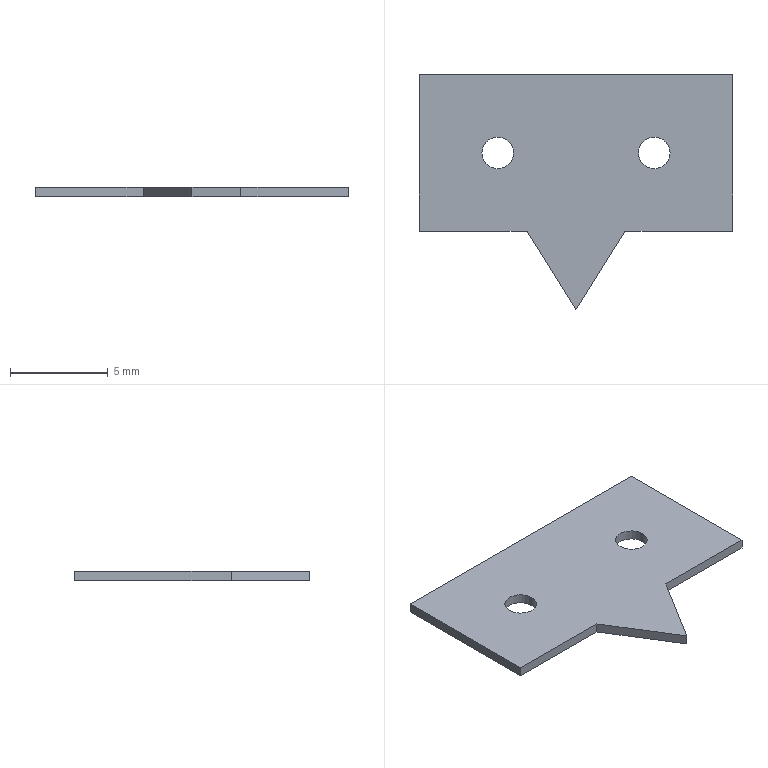Part | STEP file | 0232_012_PPS12 | 1 solid | 13 faces | box 16 x 12 x 0.5 mm | volume 66.945 mm3 | plane 9 | cylinder 4 | commonest cylinder face diameters 1.618 x4
STEP:
#1=CARTESIAN_POINT('',(0.,0.,0.));
#2=DIRECTION('',(0.,0.,1.));
#3=DIRECTION('',(1.,0.,0.));
#4=AXIS2_PLACEMENT_3D('',#1,#2,#3);
#5=CARTESIAN_POINT('',(-3.191,-4.,0.));
#6=VERTEX_POINT('',#5);
#7=CARTESIAN_POINT('',(-3.191,-4.,0.5));
#8=VERTEX_POINT('',#7);
#9=CARTESIAN_POINT('',(-3.191,-4.,0.));
#10=DIRECTION('',(0.,0.,1.));
#11=VECTOR('',#10,1.);
#12=LINE('',#9,#11);
#13=CARTESIAN_POINT('',(-4.,-4.,0.));
#14=DIRECTION('',(0.,0.,1.));
#15=DIRECTION('',(1.,0.,0.));
#16=AXIS2_PLACEMENT_3D('',#13,#14,#15);
#17=CYLINDRICAL_SURFACE('',#16,0.8088);
#18=CARTESIAN_POINT('',(6.283,0.));
#19=DIRECTION('',(0.,1.));
#20=VECTOR('',#19,1.);
#21=LINE('',#18,#20);
#22=(GEOMETRIC_REPRESENTATION_CONTEXT(2)PARAMETRIC_REPRESENTATION_CONTEXT()REPRESENTATION_CONTEXT('',''));
#23=DEFINITIONAL_REPRESENTATION('',(#21),#22);
#24=PCURVE('',#17,#23);
#25=CARTESIAN_POINT('',(-4.,-4.,0.));
#26=DIRECTION('',(0.,0.,1.));
#27=DIRECTION('',(1.,0.,0.));
#28=AXIS2_PLACEMENT_3D('',#25,#26,#27);
#29=CYLINDRICAL_SURFACE('',#28,0.8088);
#30=CARTESIAN_POINT('',(0.,0.));
#31=DIRECTION('',(0.,1.));
#32=VECTOR('',#31,1.);
#33=LINE('',#30,#32);
#34=(GEOMETRIC_REPRESENTATION_CONTEXT(2)PARAMETRIC_REPRESENTATION_CONTEXT()REPRESENTATION_CONTEXT('',''));
#35=DEFINITIONAL_REPRESENTATION('',(#33),#34);
#36=PCURVE('',#29,#35);
#37=SURFACE_CURVE('',#12,(#24,#36),.PCURVE_S1.);
#38=EDGE_CURVE('',#6,#8,#37,.T.);
#39=ORIENTED_EDGE('',*,*,#38,.T.);
#40=CARTESIAN_POINT('',(-4.809,-4.,0.5));
#41=VERTEX_POINT('',#40);
#42=CARTESIAN_POINT('',(-4.,-4.,0.5));
#43=DIRECTION('',(0.,0.,-1.));
#44=DIRECTION('',(1.,0.,0.));
#45=AXIS2_PLACEMENT_3D('',#42,#43,#44);
#46=CIRCLE('',#45,0.8088);
#47=CARTESIAN_POINT('',(6.283,0.5));
#48=DIRECTION('',(-1.,0.));
#49=VECTOR('',#48,1.);
#50=LINE('',#47,#49);
#51=(GEOMETRIC_REPRESENTATION_CONTEXT(2)PARAMETRIC_REPRESENTATION_CONTEXT()REPRESENTATION_CONTEXT('',''));
#52=DEFINITIONAL_REPRESENTATION('',(#50),#51);
#53=PCURVE('',#17,#52);
#54=CARTESIAN_POINT('',(0.,-4.698,0.5));
#55=DIRECTION('',(0.,0.,1.));
#56=DIRECTION('',(1.,0.,0.));
#57=AXIS2_PLACEMENT_3D('',#54,#55,#56);
#58=PLANE('',#57);
#59=CARTESIAN_POINT('',(-3.191,0.6981));
#60=CARTESIAN_POINT('',(-3.191,-0.7028));
#61=CARTESIAN_POINT('',(-4.404,-0.002343));
#62=CARTESIAN_POINT('',(-5.618,0.6981));
#63=CARTESIAN_POINT('',(-4.404,1.399));
#64=CARTESIAN_POINT('',(-3.191,2.099));
#65=CARTESIAN_POINT('',(-3.191,0.6981));
#66=(BOUNDED_CURVE()B_SPLINE_CURVE(2,(#59,#60,#61,#62,#63,#64,#65),.UNSPECIFIED.,.T.,.F.)B_SPLINE_CURVE_WITH_KNOTS((1,2,2,2,2,1),(-2.094,0.,2.094,4.189,6.283,8.378),.UNSPECIFIED.)CURVE()GEOMETRIC_REPRESENTATION_ITEM()RATIONAL_B_SPLINE_CURVE((1.,0.5,1.,0.5,1.,0.5,1.))REPRESENTATION_ITEM(''));
#67=(GEOMETRIC_REPRESENTATION_CONTEXT(2)PARAMETRIC_REPRESENTATION_CONTEXT()REPRESENTATION_CONTEXT('',''));
#68=DEFINITIONAL_REPRESENTATION('',(#66),#67);
#69=PCURVE('',#58,#68);
#70=SURFACE_CURVE('',#46,(#53,#69),.PCURVE_S1.);
#71=EDGE_CURVE('',#8,#41,#70,.T.);
#72=ORIENTED_EDGE('',*,*,#71,.T.);
#73=CARTESIAN_POINT('',(-4.809,-4.,0.));
#74=VERTEX_POINT('',#73);
#75=CARTESIAN_POINT('',(-4.809,-4.,0.));
#76=DIRECTION('',(0.,0.,1.));
#77=VECTOR('',#76,1.);
#78=LINE('',#75,#77);
#79=CARTESIAN_POINT('',(3.142,0.));
#80=DIRECTION('',(0.,1.));
#81=VECTOR('',#80,1.);
#82=LINE('',#79,#81);
#83=(GEOMETRIC_REPRESENTATION_CONTEXT(2)PARAMETRIC_REPRESENTATION_CONTEXT()REPRESENTATION_CONTEXT('',''));
#84=DEFINITIONAL_REPRESENTATION('',(#82),#83);
#85=PCURVE('',#17,#84);
#86=CARTESIAN_POINT('',(3.142,0.));
#87=DIRECTION('',(0.,1.));
#88=VECTOR('',#87,1.);
#89=LINE('',#86,#88);
#90=(GEOMETRIC_REPRESENTATION_CONTEXT(2)PARAMETRIC_REPRESENTATION_CONTEXT()REPRESENTATION_CONTEXT('',''));
#91=DEFINITIONAL_REPRESENTATION('',(#89),#90);
#92=PCURVE('',#29,#91);
#93=SURFACE_CURVE('',#78,(#85,#92),.PCURVE_S1.);
#94=EDGE_CURVE('',#74,#41,#93,.T.);
#95=ORIENTED_EDGE('',*,*,#94,.F.);
#96=CARTESIAN_POINT('',(-4.,-4.,0.));
#97=DIRECTION('',(0.,0.,-1.));
#98=DIRECTION('',(1.,0.,0.));
#99=AXIS2_PLACEMENT_3D('',#96,#97,#98);
#100=CIRCLE('',#99,0.8088);
#101=CARTESIAN_POINT('',(6.283,0.));
#102=DIRECTION('',(-1.,0.));
#103=VECTOR('',#102,1.);
#104=LINE('',#101,#103);
#105=(GEOMETRIC_REPRESENTATION_CONTEXT(2)PARAMETRIC_REPRESENTATION_CONTEXT()REPRESENTATION_CONTEXT('',''));
#106=DEFINITIONAL_REPRESENTATION('',(#104),#105);
#107=PCURVE('',#17,#106);
#108=CARTESIAN_POINT('',(0.,-4.698,0.));
#109=DIRECTION('',(0.,0.,1.));
#110=DIRECTION('',(1.,0.,0.));
#111=AXIS2_PLACEMENT_3D('',#108,#109,#110);
#112=PLANE('',#111);
#113=CARTESIAN_POINT('',(-3.191,0.6981));
#114=CARTESIAN_POINT('',(-3.191,-0.7028));
#115=CARTESIAN_POINT('',(-4.404,-0.002343));
#116=CARTESIAN_POINT('',(-5.618,0.6981));
#117=CARTESIAN_POINT('',(-4.404,1.399));
#118=CARTESIAN_POINT('',(-3.191,2.099));
#119=CARTESIAN_POINT('',(-3.191,0.6981));
#120=(BOUNDED_CURVE()B_SPLINE_CURVE(2,(#113,#114,#115,#116,#117,#118,#119),.UNSPECIFIED.,.T.,.F.)B_SPLINE_CURVE_WITH_KNOTS((1,2,2,2,2,1),(-2.094,0.,2.094,4.189,6.283,8.378),.UNSPECIFIED.)CURVE()GEOMETRIC_REPRESENTATION_ITEM()RATIONAL_B_SPLINE_CURVE((1.,0.5,1.,0.5,1.,0.5,1.))REPRESENTATION_ITEM(''));
#121=(GEOMETRIC_REPRESENTATION_CONTEXT(2)PARAMETRIC_REPRESENTATION_CONTEXT()REPRESENTATION_CONTEXT('',''));
#122=DEFINITIONAL_REPRESENTATION('',(#120),#121);
#123=PCURVE('',#112,#122);
#124=SURFACE_CURVE('',#100,(#107,#123),.PCURVE_S1.);
#125=EDGE_CURVE('',#6,#74,#124,.T.);
#126=ORIENTED_EDGE('',*,*,#125,.F.);
#127=EDGE_LOOP('',(#39,#72,#95,#126));
#128=FACE_BOUND('',#127,.F.);
#129=ADVANCED_FACE('',(#128),#17,.F.);
#130=CARTESIAN_POINT('',(4.809,-4.,0.));
#131=VERTEX_POINT('',#130);
#132=CARTESIAN_POINT('',(4.809,-4.,0.5));
#133=VERTEX_POINT('',#132);
#134=CARTESIAN_POINT('',(4.809,-4.,0.));
#135=DIRECTION('',(0.,0.,1.));
#136=VECTOR('',#135,1.);
#137=LINE('',#134,#136);
#138=CARTESIAN_POINT('',(4.,-4.,0.));
#139=DIRECTION('',(0.,0.,1.));
#140=DIRECTION('',(1.,0.,0.));
#141=AXIS2_PLACEMENT_3D('',#138,#139,#140);
#142=CYLINDRICAL_SURFACE('',#141,0.8088);
#143=CARTESIAN_POINT('',(6.283,0.));
#144=DIRECTION('',(0.,1.));
#145=VECTOR('',#144,1.);
#146=LINE('',#143,#145);
#147=(GEOMETRIC_REPRESENTATION_CONTEXT(2)PARAMETRIC_REPRESENTATION_CONTEXT()REPRESENTATION_CONTEXT('',''));
#148=DEFINITIONAL_REPRESENTATION('',(#146),#147);
#149=PCURVE('',#142,#148);
#150=CARTESIAN_POINT('',(4.,-4.,0.));
#151=DIRECTION('',(0.,0.,1.));
#152=DIRECTION('',(1.,0.,0.));
#153=AXIS2_PLACEMENT_3D('',#150,#151,#152);
#154=CYLINDRICAL_SURFACE('',#153,0.8088);
#155=CARTESIAN_POINT('',(0.,0.));
#156=DIRECTION('',(0.,1.));
#157=VECTOR('',#156,1.);
#158=LINE('',#155,#157);
#159=(GEOMETRIC_REPRESENTATION_CONTEXT(2)PARAMETRIC_REPRESENTATION_CONTEXT()REPRESENTATION_CONTEXT('',''));
#160=DEFINITIONAL_REPRESENTATION('',(#158),#159);
#161=PCURVE('',#154,#160);
#162=SURFACE_CURVE('',#137,(#149,#161),.PCURVE_S1.);
#163=EDGE_CURVE('',#131,#133,#162,.T.);
#164=ORIENTED_EDGE('',*,*,#163,.T.);
#165=CARTESIAN_POINT('',(3.191,-4.,0.5));
#166=VERTEX_POINT('',#165);
#167=CARTESIAN_POINT('',(4.,-4.,0.5));
#168=DIRECTION('',(0.,0.,-1.));
#169=DIRECTION('',(1.,0.,0.));
#170=AXIS2_PLACEMENT_3D('',#167,#168,#169);
#171=CIRCLE('',#170,0.8088);
#172=CARTESIAN_POINT('',(6.283,0.5));
#173=DIRECTION('',(-1.,0.));
#174=VECTOR('',#173,1.);
#175=LINE('',#172,#174);
#176=(GEOMETRIC_REPRESENTATION_CONTEXT(2)PARAMETRIC_REPRESENTATION_CONTEXT()REPRESENTATION_CONTEXT('',''));
#177=DEFINITIONAL_REPRESENTATION('',(#175),#176);
#178=PCURVE('',#142,#177);
#179=CARTESIAN_POINT('',(4.809,0.6981));
#180=CARTESIAN_POINT('',(4.809,-0.7028));
#181=CARTESIAN_POINT('',(3.596,-0.002343));
#182=CARTESIAN_POINT('',(2.382,0.6981));
#183=CARTESIAN_POINT('',(3.596,1.399));
#184=CARTESIAN_POINT('',(4.809,2.099));
#185=CARTESIAN_POINT('',(4.809,0.6981));
#186=(BOUNDED_CURVE()B_SPLINE_CURVE(2,(#179,#180,#181,#182,#183,#184,#185),.UNSPECIFIED.,.T.,.F.)B_SPLINE_CURVE_WITH_KNOTS((1,2,2,2,2,1),(-2.094,0.,2.094,4.189,6.283,8.378),.UNSPECIFIED.)CURVE()GEOMETRIC_REPRESENTATION_ITEM()RATIONAL_B_SPLINE_CURVE((1.,0.5,1.,0.5,1.,0.5,1.))REPRESENTATION_ITEM(''));
#187=(GEOMETRIC_REPRESENTATION_CONTEXT(2)PARAMETRIC_REPRESENTATION_CONTEXT()REPRESENTATION_CONTEXT('',''));
#188=DEFINITIONAL_REPRESENTATION('',(#186),#187);
#189=PCURVE('',#58,#188);
#190=SURFACE_CURVE('',#171,(#178,#189),.PCURVE_S1.);
#191=EDGE_CURVE('',#133,#166,#190,.T.);
#192=ORIENTED_EDGE('',*,*,#191,.T.);
#193=CARTESIAN_POINT('',(3.191,-4.,0.));
#194=VERTEX_POINT('',#193);
#195=CARTESIAN_POINT('',(3.191,-4.,0.));
#196=DIRECTION('',(0.,0.,1.));
#197=VECTOR('',#196,1.);
#198=LINE('',#195,#197);
#199=CARTESIAN_POINT('',(3.142,0.));
#200=DIRECTION('',(0.,1.));
#201=VECTOR('',#200,1.);
#202=LINE('',#199,#201);
#203=(GEOMETRIC_REPRESENTATION_CONTEXT(2)PARAMETRIC_REPRESENTATION_CONTEXT()REPRESENTATION_CONTEXT('',''));
#204=DEFINITIONAL_REPRESENTATION('',(#202),#203);
#205=PCURVE('',#142,#204);
#206=CARTESIAN_POINT('',(3.142,0.));
#207=DIRECTION('',(0.,1.));
#208=VECTOR('',#207,1.);
#209=LINE('',#206,#208);
#210=(GEOMETRIC_REPRESENTATION_CONTEXT(2)PARAMETRIC_REPRESENTATION_CONTEXT()REPRESENTATION_CONTEXT('',''));
#211=DEFINITIONAL_REPRESENTATION('',(#209),#210);
#212=PCURVE('',#154,#211);
#213=SURFACE_CURVE('',#198,(#205,#212),.PCURVE_S1.);
#214=EDGE_CURVE('',#194,#166,#213,.T.);
#215=ORIENTED_EDGE('',*,*,#214,.F.);
#216=CARTESIAN_POINT('',(4.,-4.,0.));
#217=DIRECTION('',(0.,0.,-1.));
#218=DIRECTION('',(1.,0.,0.));
#219=AXIS2_PLACEMENT_3D('',#216,#217,#218);
#220=CIRCLE('',#219,0.8088);
#221=CARTESIAN_POINT('',(6.283,0.));
#222=DIRECTION('',(-1.,0.));
#223=VECTOR('',#222,1.);
#224=LINE('',#221,#223);
#225=(GEOMETRIC_REPRESENTATION_CONTEXT(2)PARAMETRIC_REPRESENTATION_CONTEXT()REPRESENTATION_CONTEXT('',''));
#226=DEFINITIONAL_REPRESENTATION('',(#224),#225);
#227=PCURVE('',#142,#226);
#228=CARTESIAN_POINT('',(4.809,0.6981));
#229=CARTESIAN_POINT('',(4.809,-0.7028));
#230=CARTESIAN_POINT('',(3.596,-0.002343));
#231=CARTESIAN_POINT('',(2.382,0.6981));
#232=CARTESIAN_POINT('',(3.596,1.399));
#233=CARTESIAN_POINT('',(4.809,2.099));
#234=CARTESIAN_POINT('',(4.809,0.6981));
#235=(BOUNDED_CURVE()B_SPLINE_CURVE(2,(#228,#229,#230,#231,#232,#233,#234),.UNSPECIFIED.,.T.,.F.)B_SPLINE_CURVE_WITH_KNOTS((1,2,2,2,2,1),(-2.094,0.,2.094,4.189,6.283,8.378),.UNSPECIFIED.)CURVE()GEOMETRIC_REPRESENTATION_ITEM()RATIONAL_B_SPLINE_CURVE((1.,0.5,1.,0.5,1.,0.5,1.))REPRESENTATION_ITEM(''));
#236=(GEOMETRIC_REPRESENTATION_CONTEXT(2)PARAMETRIC_REPRESENTATION_CONTEXT()REPRESENTATION_CONTEXT('',''));
#237=DEFINITIONAL_REPRESENTATION('',(#235),#236);
#238=PCURVE('',#112,#237);
#239=SURFACE_CURVE('',#220,(#227,#238),.PCURVE_S1.);
#240=EDGE_CURVE('',#131,#194,#239,.T.);
#241=ORIENTED_EDGE('',*,*,#240,.F.);
#242=EDGE_LOOP('',(#164,#192,#215,#241));
#243=FACE_BOUND('',#242,.F.);
#244=ADVANCED_FACE('',(#243),#142,.F.);
#245=ORIENTED_EDGE('',*,*,#125,.F.);
#246=CARTESIAN_POINT('',(-4.,-4.,0.));
#247=DIRECTION('',(0.,0.,-1.));
#248=DIRECTION('',(1.,0.,0.));
#249=AXIS2_PLACEMENT_3D('',#246,#247,#248);
#250=CIRCLE('',#249,0.8088);
#251=CARTESIAN_POINT('',(-3.191,0.6981));
#252=CARTESIAN_POINT('',(-3.191,-0.7028));
#253=CARTESIAN_POINT('',(-4.404,-0.002343));
#254=CARTESIAN_POINT('',(-5.618,0.6981));
#255=CARTESIAN_POINT('',(-4.404,1.399));
#256=CARTESIAN_POINT('',(-3.191,2.099));
#257=CARTESIAN_POINT('',(-3.191,0.6981));
#258=(BOUNDED_CURVE()B_SPLINE_CURVE(2,(#251,#252,#253,#254,#255,#256,#257),.UNSPECIFIED.,.T.,.F.)B_SPLINE_CURVE_WITH_KNOTS((1,2,2,2,2,1),(-2.094,0.,2.094,4.189,6.283,8.378),.UNSPECIFIED.)CURVE()GEOMETRIC_REPRESENTATION_ITEM()RATIONAL_B_SPLINE_CURVE((1.,0.5,1.,0.5,1.,0.5,1.))REPRESENTATION_ITEM(''));
#259=(GEOMETRIC_REPRESENTATION_CONTEXT(2)PARAMETRIC_REPRESENTATION_CONTEXT()REPRESENTATION_CONTEXT('',''));
#260=DEFINITIONAL_REPRESENTATION('',(#258),#259);
#261=PCURVE('',#112,#260);
#262=CARTESIAN_POINT('',(6.283,0.));
#263=DIRECTION('',(-1.,0.));
#264=VECTOR('',#263,1.);
#265=LINE('',#262,#264);
#266=(GEOMETRIC_REPRESENTATION_CONTEXT(2)PARAMETRIC_REPRESENTATION_CONTEXT()REPRESENTATION_CONTEXT('',''));
#267=DEFINITIONAL_REPRESENTATION('',(#265),#266);
#268=PCURVE('',#29,#267);
#269=SURFACE_CURVE('',#250,(#261,#268),.PCURVE_S1.);
#270=EDGE_CURVE('',#74,#6,#269,.T.);
#271=ORIENTED_EDGE('',*,*,#270,.F.);
#272=EDGE_LOOP('',(#245,#271));
#273=FACE_BOUND('',#272,.T.);
#274=ORIENTED_EDGE('',*,*,#240,.F.);
#275=CARTESIAN_POINT('',(4.,-4.,0.));
#276=DIRECTION('',(0.,0.,-1.));
#277=DIRECTION('',(1.,0.,0.));
#278=AXIS2_PLACEMENT_3D('',#275,#276,#277);
#279=CIRCLE('',#278,0.8088);
#280=CARTESIAN_POINT('',(4.809,0.6981));
#281=CARTESIAN_POINT('',(4.809,-0.7028));
#282=CARTESIAN_POINT('',(3.596,-0.002343));
#283=CARTESIAN_POINT('',(2.382,0.6981));
#284=CARTESIAN_POINT('',(3.596,1.399));
#285=CARTESIAN_POINT('',(4.809,2.099));
#286=CARTESIAN_POINT('',(4.809,0.6981));
#287=(BOUNDED_CURVE()B_SPLINE_CURVE(2,(#280,#281,#282,#283,#284,#285,#286),.UNSPECIFIED.,.T.,.F.)B_SPLINE_CURVE_WITH_KNOTS((1,2,2,2,2,1),(-2.094,0.,2.094,4.189,6.283,8.378),.UNSPECIFIED.)CURVE()GEOMETRIC_REPRESENTATION_ITEM()RATIONAL_B_SPLINE_CURVE((1.,0.5,1.,0.5,1.,0.5,1.))REPRESENTATION_ITEM(''));
#288=(GEOMETRIC_REPRESENTATION_CONTEXT(2)PARAMETRIC_REPRESENTATION_CONTEXT()REPRESENTATION_CONTEXT('',''));
#289=DEFINITIONAL_REPRESENTATION('',(#287),#288);
#290=PCURVE('',#112,#289);
#291=CARTESIAN_POINT('',(6.283,0.));
#292=DIRECTION('',(-1.,0.));
#293=VECTOR('',#292,1.);
#294=LINE('',#291,#293);
#295=(GEOMETRIC_REPRESENTATION_CONTEXT(2)PARAMETRIC_REPRESENTATION_CONTEXT()REPRESENTATION_CONTEXT('',''));
#296=DEFINITIONAL_REPRESENTATION('',(#294),#295);
#297=PCURVE('',#154,#296);
#298=SURFACE_CURVE('',#279,(#290,#297),.PCURVE_S1.);
#299=EDGE_CURVE('',#194,#131,#298,.T.);
#300=ORIENTED_EDGE('',*,*,#299,.F.);
#301=EDGE_LOOP('',(#274,#300));
#302=FACE_BOUND('',#301,.T.);
#303=CARTESIAN_POINT('',(-8.,0.,0.));
#304=VERTEX_POINT('',#303);
#305=CARTESIAN_POINT('',(-8.,-8.,0.));
#306=VERTEX_POINT('',#305);
#307=CARTESIAN_POINT('',(-8.,-4.698,0.));
#308=DIRECTION('',(0.,-1.,0.));
#309=VECTOR('',#308,1.);
#310=LINE('',#307,#309);
#311=CARTESIAN_POINT('',(-8.,0.));
#312=DIRECTION('',(0.,-1.));
#313=VECTOR('',#312,1.);
#314=LINE('',#311,#313);
#315=(GEOMETRIC_REPRESENTATION_CONTEXT(2)PARAMETRIC_REPRESENTATION_CONTEXT()REPRESENTATION_CONTEXT('',''));
#316=DEFINITIONAL_REPRESENTATION('',(#314),#315);
#317=PCURVE('',#112,#316);
#318=CARTESIAN_POINT('',(-8.,-8.,0.));
#319=DIRECTION('',(-1.,0.,0.));
#320=DIRECTION('',(0.,0.,1.));
#321=AXIS2_PLACEMENT_3D('',#318,#319,#320);
#322=PLANE('',#321);
#323=CARTESIAN_POINT('',(0.,3.302));
#324=DIRECTION('',(0.,-1.));
#325=VECTOR('',#324,1.);
#326=LINE('',#323,#325);
#327=(GEOMETRIC_REPRESENTATION_CONTEXT(2)PARAMETRIC_REPRESENTATION_CONTEXT()REPRESENTATION_CONTEXT('',''));
#328=DEFINITIONAL_REPRESENTATION('',(#326),#327);
#329=PCURVE('',#322,#328);
#330=SURFACE_CURVE('',#310,(#317,#329),.PCURVE_S1.);
#331=EDGE_CURVE('',#304,#306,#330,.T.);
#332=ORIENTED_EDGE('',*,*,#331,.F.);
#333=CARTESIAN_POINT('',(8.,0.,0.));
#334=VERTEX_POINT('',#333);
#335=CARTESIAN_POINT('',(0.,0.,0.));
#336=DIRECTION('',(-1.,0.,0.));
#337=VECTOR('',#336,1.);
#338=LINE('',#335,#337);
#339=CARTESIAN_POINT('',(0.,4.698));
#340=DIRECTION('',(-1.,0.));
#341=VECTOR('',#340,1.);
#342=LINE('',#339,#341);
#343=(GEOMETRIC_REPRESENTATION_CONTEXT(2)PARAMETRIC_REPRESENTATION_CONTEXT()REPRESENTATION_CONTEXT('',''));
#344=DEFINITIONAL_REPRESENTATION('',(#342),#343);
#345=PCURVE('',#112,#344);
#346=CARTESIAN_POINT('',(-8.,0.,0.));
#347=DIRECTION('',(0.,1.,0.));
#348=DIRECTION('',(0.,0.,1.));
#349=AXIS2_PLACEMENT_3D('',#346,#347,#348);
#350=PLANE('',#349);
#351=CARTESIAN_POINT('',(0.,8.));
#352=DIRECTION('',(0.,-1.));
#353=VECTOR('',#352,1.);
#354=LINE('',#351,#353);
#355=(GEOMETRIC_REPRESENTATION_CONTEXT(2)PARAMETRIC_REPRESENTATION_CONTEXT()REPRESENTATION_CONTEXT('',''));
#356=DEFINITIONAL_REPRESENTATION('',(#354),#355);
#357=PCURVE('',#350,#356);
#358=SURFACE_CURVE('',#338,(#345,#357),.PCURVE_S1.);
#359=EDGE_CURVE('',#334,#304,#358,.T.);
#360=ORIENTED_EDGE('',*,*,#359,.F.);
#361=CARTESIAN_POINT('',(8.,-8.,0.));
#362=VERTEX_POINT('',#361);
#363=CARTESIAN_POINT('',(8.,-4.698,0.));
#364=DIRECTION('',(0.,1.,0.));
#365=VECTOR('',#364,1.);
#366=LINE('',#363,#365);
#367=CARTESIAN_POINT('',(8.,0.));
#368=DIRECTION('',(0.,1.));
#369=VECTOR('',#368,1.);
#370=LINE('',#367,#369);
#371=(GEOMETRIC_REPRESENTATION_CONTEXT(2)PARAMETRIC_REPRESENTATION_CONTEXT()REPRESENTATION_CONTEXT('',''));
#372=DEFINITIONAL_REPRESENTATION('',(#370),#371);
#373=PCURVE('',#112,#372);
#374=CARTESIAN_POINT('',(8.,0.,0.));
#375=DIRECTION('',(1.,0.,0.));
#376=DIRECTION('',(0.,0.,-1.));
#377=AXIS2_PLACEMENT_3D('',#374,#375,#376);
#378=PLANE('',#377);
#379=CARTESIAN_POINT('',(0.,-4.698));
#380=DIRECTION('',(0.,1.));
#381=VECTOR('',#380,1.);
#382=LINE('',#379,#381);
#383=(GEOMETRIC_REPRESENTATION_CONTEXT(2)PARAMETRIC_REPRESENTATION_CONTEXT()REPRESENTATION_CONTEXT('',''));
#384=DEFINITIONAL_REPRESENTATION('',(#382),#383);
#385=PCURVE('',#378,#384);
#386=SURFACE_CURVE('',#366,(#373,#385),.PCURVE_S1.);
#387=EDGE_CURVE('',#362,#334,#386,.T.);
#388=ORIENTED_EDGE('',*,*,#387,.F.);
#389=CARTESIAN_POINT('',(2.5,-8.,0.));
#390=VERTEX_POINT('',#389);
#391=CARTESIAN_POINT('',(0.,-8.,0.));
#392=DIRECTION('',(1.,0.,0.));
#393=VECTOR('',#392,1.);
#394=LINE('',#391,#393);
#395=CARTESIAN_POINT('',(0.,-3.302));
#396=DIRECTION('',(1.,0.));
#397=VECTOR('',#396,1.);
#398=LINE('',#395,#397);
#399=(GEOMETRIC_REPRESENTATION_CONTEXT(2)PARAMETRIC_REPRESENTATION_CONTEXT()REPRESENTATION_CONTEXT('',''));
#400=DEFINITIONAL_REPRESENTATION('',(#398),#399);
#401=PCURVE('',#112,#400);
#402=CARTESIAN_POINT('',(8.,-8.,0.));
#403=DIRECTION('',(0.,-1.,0.));
#404=DIRECTION('',(0.,0.,-1.));
#405=AXIS2_PLACEMENT_3D('',#402,#403,#404);
#406=PLANE('',#405);
#407=CARTESIAN_POINT('',(0.,-8.));
#408=DIRECTION('',(0.,1.));
#409=VECTOR('',#408,1.);
#410=LINE('',#407,#409);
#411=(GEOMETRIC_REPRESENTATION_CONTEXT(2)PARAMETRIC_REPRESENTATION_CONTEXT()REPRESENTATION_CONTEXT('',''));
#412=DEFINITIONAL_REPRESENTATION('',(#410),#411);
#413=PCURVE('',#406,#412);
#414=SURFACE_CURVE('',#394,(#401,#413),.PCURVE_S1.);
#415=EDGE_CURVE('',#390,#362,#414,.T.);
#416=ORIENTED_EDGE('',*,*,#415,.F.);
#417=CARTESIAN_POINT('',(0.,-12.,0.));
#418=VERTEX_POINT('',#417);
#419=CARTESIAN_POINT('',(0.,-12.,0.));
#420=DIRECTION('',(0.53,0.848,0.));
#421=VECTOR('',#420,1.);
#422=LINE('',#419,#421);
#423=CARTESIAN_POINT('',(0.,-7.302));
#424=DIRECTION('',(0.53,0.848));
#425=VECTOR('',#424,1.);
#426=LINE('',#423,#425);
#427=(GEOMETRIC_REPRESENTATION_CONTEXT(2)PARAMETRIC_REPRESENTATION_CONTEXT()REPRESENTATION_CONTEXT('',''));
#428=DEFINITIONAL_REPRESENTATION('',(#426),#427);
#429=PCURVE('',#112,#428);
#430=CARTESIAN_POINT('',(2.5,-8.,0.));
#431=DIRECTION('',(0.848,-0.53,0.));
#432=DIRECTION('',(0.53,0.848,0.));
#433=AXIS2_PLACEMENT_3D('',#430,#431,#432);
#434=PLANE('',#433);
#435=CARTESIAN_POINT('',(-4.717,0.));
#436=DIRECTION('',(1.,0.));
#437=VECTOR('',#436,1.);
#438=LINE('',#435,#437);
#439=(GEOMETRIC_REPRESENTATION_CONTEXT(2)PARAMETRIC_REPRESENTATION_CONTEXT()REPRESENTATION_CONTEXT('',''));
#440=DEFINITIONAL_REPRESENTATION('',(#438),#439);
#441=PCURVE('',#434,#440);
#442=SURFACE_CURVE('',#422,(#429,#441),.PCURVE_S1.);
#443=EDGE_CURVE('',#418,#390,#442,.T.);
#444=ORIENTED_EDGE('',*,*,#443,.F.);
#445=CARTESIAN_POINT('',(-2.5,-8.,0.));
#446=VERTEX_POINT('',#445);
#447=CARTESIAN_POINT('',(-2.5,-8.,0.));
#448=DIRECTION('',(0.53,-0.848,0.));
#449=VECTOR('',#448,1.);
#450=LINE('',#447,#449);
#451=CARTESIAN_POINT('',(-2.5,-3.302));
#452=DIRECTION('',(0.53,-0.848));
#453=VECTOR('',#452,1.);
#454=LINE('',#451,#453);
#455=(GEOMETRIC_REPRESENTATION_CONTEXT(2)PARAMETRIC_REPRESENTATION_CONTEXT()REPRESENTATION_CONTEXT('',''));
#456=DEFINITIONAL_REPRESENTATION('',(#454),#455);
#457=PCURVE('',#112,#456);
#458=CARTESIAN_POINT('',(0.,-12.,0.));
#459=DIRECTION('',(-0.848,-0.53,0.));
#460=DIRECTION('',(0.53,-0.848,0.));
#461=AXIS2_PLACEMENT_3D('',#458,#459,#460);
#462=PLANE('',#461);
#463=CARTESIAN_POINT('',(-4.717,0.));
#464=DIRECTION('',(1.,0.));
#465=VECTOR('',#464,1.);
#466=LINE('',#463,#465);
#467=(GEOMETRIC_REPRESENTATION_CONTEXT(2)PARAMETRIC_REPRESENTATION_CONTEXT()REPRESENTATION_CONTEXT('',''));
#468=DEFINITIONAL_REPRESENTATION('',(#466),#467);
#469=PCURVE('',#462,#468);
#470=SURFACE_CURVE('',#450,(#457,#469),.PCURVE_S1.);
#471=EDGE_CURVE('',#446,#418,#470,.T.);
#472=ORIENTED_EDGE('',*,*,#471,.F.);
#473=CARTESIAN_POINT('',(0.,-8.,0.));
#474=DIRECTION('',(1.,0.,0.));
#475=VECTOR('',#474,1.);
#476=LINE('',#473,#475);
#477=CARTESIAN_POINT('',(0.,-3.302));
#478=DIRECTION('',(1.,0.));
#479=VECTOR('',#478,1.);
#480=LINE('',#477,#479);
#481=(GEOMETRIC_REPRESENTATION_CONTEXT(2)PARAMETRIC_REPRESENTATION_CONTEXT()REPRESENTATION_CONTEXT('',''));
#482=DEFINITIONAL_REPRESENTATION('',(#480),#481);
#483=PCURVE('',#112,#482);
#484=CARTESIAN_POINT('',(-2.5,-8.,0.));
#485=DIRECTION('',(0.,-1.,0.));
#486=DIRECTION('',(0.,0.,-1.));
#487=AXIS2_PLACEMENT_3D('',#484,#485,#486);
#488=PLANE('',#487);
#489=CARTESIAN_POINT('',(0.,2.5));
#490=DIRECTION('',(0.,1.));
#491=VECTOR('',#490,1.);
#492=LINE('',#489,#491);
#493=(GEOMETRIC_REPRESENTATION_CONTEXT(2)PARAMETRIC_REPRESENTATION_CONTEXT()REPRESENTATION_CONTEXT('',''));
#494=DEFINITIONAL_REPRESENTATION('',(#492),#493);
#495=PCURVE('',#488,#494);
#496=SURFACE_CURVE('',#476,(#483,#495),.PCURVE_S1.);
#497=EDGE_CURVE('',#306,#446,#496,.T.);
#498=ORIENTED_EDGE('',*,*,#497,.F.);
#499=EDGE_LOOP('',(#332,#360,#388,#416,#444,#472,#498));
#500=FACE_BOUND('',#499,.T.);
#501=ADVANCED_FACE('',(#273,#302,#500),#112,.F.);
#502=CARTESIAN_POINT('',(-4.,-4.,0.5));
#503=DIRECTION('',(0.,0.,-1.));
#504=DIRECTION('',(1.,0.,0.));
#505=AXIS2_PLACEMENT_3D('',#502,#503,#504);
#506=CIRCLE('',#505,0.8088);
#507=CARTESIAN_POINT('',(6.283,0.5));
#508=DIRECTION('',(-1.,0.));
#509=VECTOR('',#508,1.);
#510=LINE('',#507,#509);
#511=(GEOMETRIC_REPRESENTATION_CONTEXT(2)PARAMETRIC_REPRESENTATION_CONTEXT()REPRESENTATION_CONTEXT('',''));
#512=DEFINITIONAL_REPRESENTATION('',(#510),#511);
#513=PCURVE('',#29,#512);
#514=CARTESIAN_POINT('',(-3.191,0.6981));
#515=CARTESIAN_POINT('',(-3.191,-0.7028));
#516=CARTESIAN_POINT('',(-4.404,-0.002343));
#517=CARTESIAN_POINT('',(-5.618,0.6981));
#518=CARTESIAN_POINT('',(-4.404,1.399));
#519=CARTESIAN_POINT('',(-3.191,2.099));
#520=CARTESIAN_POINT('',(-3.191,0.6981));
#521=(BOUNDED_CURVE()B_SPLINE_CURVE(2,(#514,#515,#516,#517,#518,#519,#520),.UNSPECIFIED.,.T.,.F.)B_SPLINE_CURVE_WITH_KNOTS((1,2,2,2,2,1),(-2.094,0.,2.094,4.189,6.283,8.378),.UNSPECIFIED.)CURVE()GEOMETRIC_REPRESENTATION_ITEM()RATIONAL_B_SPLINE_CURVE((1.,0.5,1.,0.5,1.,0.5,1.))REPRESENTATION_ITEM(''));
#522=(GEOMETRIC_REPRESENTATION_CONTEXT(2)PARAMETRIC_REPRESENTATION_CONTEXT()REPRESENTATION_CONTEXT('',''));
#523=DEFINITIONAL_REPRESENTATION('',(#521),#522);
#524=PCURVE('',#58,#523);
#525=SURFACE_CURVE('',#506,(#513,#524),.PCURVE_S1.);
#526=EDGE_CURVE('',#41,#8,#525,.T.);
#527=ORIENTED_EDGE('',*,*,#526,.T.);
#528=ORIENTED_EDGE('',*,*,#38,.F.);
#529=ORIENTED_EDGE('',*,*,#270,.F.);
#530=ORIENTED_EDGE('',*,*,#94,.T.);
#531=EDGE_LOOP('',(#527,#528,#529,#530));
#532=FACE_BOUND('',#531,.F.);
#533=ADVANCED_FACE('',(#532),#29,.F.);
#534=CARTESIAN_POINT('',(4.,-4.,0.5));
#535=DIRECTION('',(0.,0.,-1.));
#536=DIRECTION('',(1.,0.,0.));
#537=AXIS2_PLACEMENT_3D('',#534,#535,#536);
#538=CIRCLE('',#537,0.8088);
#539=CARTESIAN_POINT('',(6.283,0.5));
#540=DIRECTION('',(-1.,0.));
#541=VECTOR('',#540,1.);
#542=LINE('',#539,#541);
#543=(GEOMETRIC_REPRESENTATION_CONTEXT(2)PARAMETRIC_REPRESENTATION_CONTEXT()REPRESENTATION_CONTEXT('',''));
#544=DEFINITIONAL_REPRESENTATION('',(#542),#543);
#545=PCURVE('',#154,#544);
#546=CARTESIAN_POINT('',(4.809,0.6981));
#547=CARTESIAN_POINT('',(4.809,-0.7028));
#548=CARTESIAN_POINT('',(3.596,-0.002343));
#549=CARTESIAN_POINT('',(2.382,0.6981));
#550=CARTESIAN_POINT('',(3.596,1.399));
#551=CARTESIAN_POINT('',(4.809,2.099));
#552=CARTESIAN_POINT('',(4.809,0.6981));
#553=(BOUNDED_CURVE()B_SPLINE_CURVE(2,(#546,#547,#548,#549,#550,#551,#552),.UNSPECIFIED.,.T.,.F.)B_SPLINE_CURVE_WITH_KNOTS((1,2,2,2,2,1),(-2.094,0.,2.094,4.189,6.283,8.378),.UNSPECIFIED.)CURVE()GEOMETRIC_REPRESENTATION_ITEM()RATIONAL_B_SPLINE_CURVE((1.,0.5,1.,0.5,1.,0.5,1.))REPRESENTATION_ITEM(''));
#554=(GEOMETRIC_REPRESENTATION_CONTEXT(2)PARAMETRIC_REPRESENTATION_CONTEXT()REPRESENTATION_CONTEXT('',''));
#555=DEFINITIONAL_REPRESENTATION('',(#553),#554);
#556=PCURVE('',#58,#555);
#557=SURFACE_CURVE('',#538,(#545,#556),.PCURVE_S1.);
#558=EDGE_CURVE('',#166,#133,#557,.T.);
#559=ORIENTED_EDGE('',*,*,#558,.T.);
#560=ORIENTED_EDGE('',*,*,#163,.F.);
#561=ORIENTED_EDGE('',*,*,#299,.F.);
#562=ORIENTED_EDGE('',*,*,#214,.T.);
#563=EDGE_LOOP('',(#559,#560,#561,#562));
#564=FACE_BOUND('',#563,.F.);
#565=ADVANCED_FACE('',(#564),#154,.F.);
#566=ORIENTED_EDGE('',*,*,#497,.T.);
#567=CARTESIAN_POINT('',(-2.5,-8.,0.5));
#568=VERTEX_POINT('',#567);
#569=CARTESIAN_POINT('',(-2.5,-8.,0.));
#570=DIRECTION('',(0.,0.,1.));
#571=VECTOR('',#570,1.);
#572=LINE('',#569,#571);
#573=CARTESIAN_POINT('',(0.,0.));
#574=DIRECTION('',(-1.,0.));
#575=VECTOR('',#574,1.);
#576=LINE('',#573,#575);
#577=(GEOMETRIC_REPRESENTATION_CONTEXT(2)PARAMETRIC_REPRESENTATION_CONTEXT()REPRESENTATION_CONTEXT('',''));
#578=DEFINITIONAL_REPRESENTATION('',(#576),#577);
#579=PCURVE('',#488,#578);
#580=CARTESIAN_POINT('',(-4.717,0.));
#581=DIRECTION('',(0.,1.));
#582=VECTOR('',#581,1.);
#583=LINE('',#580,#582);
#584=(GEOMETRIC_REPRESENTATION_CONTEXT(2)PARAMETRIC_REPRESENTATION_CONTEXT()REPRESENTATION_CONTEXT('',''));
#585=DEFINITIONAL_REPRESENTATION('',(#583),#584);
#586=PCURVE('',#462,#585);
#587=SURFACE_CURVE('',#572,(#579,#586),.PCURVE_S1.);
#588=EDGE_CURVE('',#446,#568,#587,.T.);
#589=ORIENTED_EDGE('',*,*,#588,.T.);
#590=CARTESIAN_POINT('',(-8.,-8.,0.5));
#591=VERTEX_POINT('',#590);
#592=CARTESIAN_POINT('',(-2.5,-8.,0.5));
#593=DIRECTION('',(-1.,0.,0.));
#594=VECTOR('',#593,1.);
#595=LINE('',#592,#594);
#596=CARTESIAN_POINT('',(-0.5,0.));
#597=DIRECTION('',(0.,-1.));
#598=VECTOR('',#597,1.);
#599=LINE('',#596,#598);
#600=(GEOMETRIC_REPRESENTATION_CONTEXT(2)PARAMETRIC_REPRESENTATION_CONTEXT()REPRESENTATION_CONTEXT('',''));
#601=DEFINITIONAL_REPRESENTATION('',(#599),#600);
#602=PCURVE('',#488,#601);
#603=CARTESIAN_POINT('',(-2.5,-3.302));
#604=DIRECTION('',(-1.,0.));
#605=VECTOR('',#604,1.);
#606=LINE('',#603,#605);
#607=(GEOMETRIC_REPRESENTATION_CONTEXT(2)PARAMETRIC_REPRESENTATION_CONTEXT()REPRESENTATION_CONTEXT('',''));
#608=DEFINITIONAL_REPRESENTATION('',(#606),#607);
#609=PCURVE('',#58,#608);
#610=SURFACE_CURVE('',#595,(#602,#609),.PCURVE_S1.);
#611=EDGE_CURVE('',#568,#591,#610,.T.);
#612=ORIENTED_EDGE('',*,*,#611,.T.);
#613=CARTESIAN_POINT('',(-8.,-8.,0.));
#614=DIRECTION('',(0.,0.,-1.));
#615=VECTOR('',#614,1.);
#616=LINE('',#613,#615);
#617=CARTESIAN_POINT('',(0.,-5.5));
#618=DIRECTION('',(1.,0.));
#619=VECTOR('',#618,1.);
#620=LINE('',#617,#619);
#621=(GEOMETRIC_REPRESENTATION_CONTEXT(2)PARAMETRIC_REPRESENTATION_CONTEXT()REPRESENTATION_CONTEXT('',''));
#622=DEFINITIONAL_REPRESENTATION('',(#620),#621);
#623=PCURVE('',#488,#622);
#624=CARTESIAN_POINT('',(0.,0.));
#625=DIRECTION('',(-1.,0.));
#626=VECTOR('',#625,1.);
#627=LINE('',#624,#626);
#628=(GEOMETRIC_REPRESENTATION_CONTEXT(2)PARAMETRIC_REPRESENTATION_CONTEXT()REPRESENTATION_CONTEXT('',''));
#629=DEFINITIONAL_REPRESENTATION('',(#627),#628);
#630=PCURVE('',#322,#629);
#631=SURFACE_CURVE('',#616,(#623,#630),.PCURVE_S1.);
#632=EDGE_CURVE('',#591,#306,#631,.T.);
#633=ORIENTED_EDGE('',*,*,#632,.T.);
#634=EDGE_LOOP('',(#566,#589,#612,#633));
#635=FACE_BOUND('',#634,.T.);
#636=ADVANCED_FACE('',(#635),#488,.T.);
#637=ORIENTED_EDGE('',*,*,#331,.T.);
#638=ORIENTED_EDGE('',*,*,#632,.F.);
#639=CARTESIAN_POINT('',(-8.,0.,0.5));
#640=VERTEX_POINT('',#639);
#641=CARTESIAN_POINT('',(-8.,-8.,0.5));
#642=DIRECTION('',(0.,1.,0.));
#643=VECTOR('',#642,1.);
#644=LINE('',#641,#643);
#645=CARTESIAN_POINT('',(0.5,0.));
#646=DIRECTION('',(0.,1.));
#647=VECTOR('',#646,1.);
#648=LINE('',#645,#647);
#649=(GEOMETRIC_REPRESENTATION_CONTEXT(2)PARAMETRIC_REPRESENTATION_CONTEXT()REPRESENTATION_CONTEXT('',''));
#650=DEFINITIONAL_REPRESENTATION('',(#648),#649);
#651=PCURVE('',#322,#650);
#652=CARTESIAN_POINT('',(-8.,-3.302));
#653=DIRECTION('',(0.,1.));
#654=VECTOR('',#653,1.);
#655=LINE('',#652,#654);
#656=(GEOMETRIC_REPRESENTATION_CONTEXT(2)PARAMETRIC_REPRESENTATION_CONTEXT()REPRESENTATION_CONTEXT('',''));
#657=DEFINITIONAL_REPRESENTATION('',(#655),#656);
#658=PCURVE('',#58,#657);
#659=SURFACE_CURVE('',#644,(#651,#658),.PCURVE_S1.);
#660=EDGE_CURVE('',#591,#640,#659,.T.);
#661=ORIENTED_EDGE('',*,*,#660,.T.);
#662=CARTESIAN_POINT('',(-8.,0.,0.));
#663=DIRECTION('',(0.,0.,-1.));
#664=VECTOR('',#663,1.);
#665=LINE('',#662,#664);
#666=CARTESIAN_POINT('',(0.,8.));
#667=DIRECTION('',(-1.,0.));
#668=VECTOR('',#667,1.);
#669=LINE('',#666,#668);
#670=(GEOMETRIC_REPRESENTATION_CONTEXT(2)PARAMETRIC_REPRESENTATION_CONTEXT()REPRESENTATION_CONTEXT('',''));
#671=DEFINITIONAL_REPRESENTATION('',(#669),#670);
#672=PCURVE('',#322,#671);
#673=CARTESIAN_POINT('',(0.,0.));
#674=DIRECTION('',(-1.,0.));
#675=VECTOR('',#674,1.);
#676=LINE('',#673,#675);
#677=(GEOMETRIC_REPRESENTATION_CONTEXT(2)PARAMETRIC_REPRESENTATION_CONTEXT()REPRESENTATION_CONTEXT('',''));
#678=DEFINITIONAL_REPRESENTATION('',(#676),#677);
#679=PCURVE('',#350,#678);
#680=SURFACE_CURVE('',#665,(#672,#679),.PCURVE_S1.);
#681=EDGE_CURVE('',#640,#304,#680,.T.);
#682=ORIENTED_EDGE('',*,*,#681,.T.);
#683=EDGE_LOOP('',(#637,#638,#661,#682));
#684=FACE_BOUND('',#683,.T.);
#685=ADVANCED_FACE('',(#684),#322,.T.);
#686=ORIENTED_EDGE('',*,*,#359,.T.);
#687=ORIENTED_EDGE('',*,*,#681,.F.);
#688=CARTESIAN_POINT('',(8.,0.,0.5));
#689=VERTEX_POINT('',#688);
#690=CARTESIAN_POINT('',(-8.,0.,0.5));
#691=DIRECTION('',(1.,0.,0.));
#692=VECTOR('',#691,1.);
#693=LINE('',#690,#692);
#694=CARTESIAN_POINT('',(0.5,0.));
#695=DIRECTION('',(0.,1.));
#696=VECTOR('',#695,1.);
#697=LINE('',#694,#696);
#698=(GEOMETRIC_REPRESENTATION_CONTEXT(2)PARAMETRIC_REPRESENTATION_CONTEXT()REPRESENTATION_CONTEXT('',''));
#699=DEFINITIONAL_REPRESENTATION('',(#697),#698);
#700=PCURVE('',#350,#699);
#701=CARTESIAN_POINT('',(-8.,4.698));
#702=DIRECTION('',(1.,0.));
#703=VECTOR('',#702,1.);
#704=LINE('',#701,#703);
#705=(GEOMETRIC_REPRESENTATION_CONTEXT(2)PARAMETRIC_REPRESENTATION_CONTEXT()REPRESENTATION_CONTEXT('',''));
#706=DEFINITIONAL_REPRESENTATION('',(#704),#705);
#707=PCURVE('',#58,#706);
#708=SURFACE_CURVE('',#693,(#700,#707),.PCURVE_S1.);
#709=EDGE_CURVE('',#640,#689,#708,.T.);
#710=ORIENTED_EDGE('',*,*,#709,.T.);
#711=CARTESIAN_POINT('',(8.,0.,0.));
#712=DIRECTION('',(0.,0.,-1.));
#713=VECTOR('',#712,1.);
#714=LINE('',#711,#713);
#715=CARTESIAN_POINT('',(0.,16.));
#716=DIRECTION('',(-1.,0.));
#717=VECTOR('',#716,1.);
#718=LINE('',#715,#717);
#719=(GEOMETRIC_REPRESENTATION_CONTEXT(2)PARAMETRIC_REPRESENTATION_CONTEXT()REPRESENTATION_CONTEXT('',''));
#720=DEFINITIONAL_REPRESENTATION('',(#718),#719);
#721=PCURVE('',#350,#720);
#722=CARTESIAN_POINT('',(0.,0.));
#723=DIRECTION('',(1.,0.));
#724=VECTOR('',#723,1.);
#725=LINE('',#722,#724);
#726=(GEOMETRIC_REPRESENTATION_CONTEXT(2)PARAMETRIC_REPRESENTATION_CONTEXT()REPRESENTATION_CONTEXT('',''));
#727=DEFINITIONAL_REPRESENTATION('',(#725),#726);
#728=PCURVE('',#378,#727);
#729=SURFACE_CURVE('',#714,(#721,#728),.PCURVE_S1.);
#730=EDGE_CURVE('',#689,#334,#729,.T.);
#731=ORIENTED_EDGE('',*,*,#730,.T.);
#732=EDGE_LOOP('',(#686,#687,#710,#731));
#733=FACE_BOUND('',#732,.T.);
#734=ADVANCED_FACE('',(#733),#350,.T.);
#735=ORIENTED_EDGE('',*,*,#387,.T.);
#736=ORIENTED_EDGE('',*,*,#730,.F.);
#737=CARTESIAN_POINT('',(8.,-8.,0.5));
#738=VERTEX_POINT('',#737);
#739=CARTESIAN_POINT('',(8.,0.,0.5));
#740=DIRECTION('',(0.,-1.,0.));
#741=VECTOR('',#740,1.);
#742=LINE('',#739,#741);
#743=CARTESIAN_POINT('',(-0.5,0.));
#744=DIRECTION('',(0.,-1.));
#745=VECTOR('',#744,1.);
#746=LINE('',#743,#745);
#747=(GEOMETRIC_REPRESENTATION_CONTEXT(2)PARAMETRIC_REPRESENTATION_CONTEXT()REPRESENTATION_CONTEXT('',''));
#748=DEFINITIONAL_REPRESENTATION('',(#746),#747);
#749=PCURVE('',#378,#748);
#750=CARTESIAN_POINT('',(8.,4.698));
#751=DIRECTION('',(0.,-1.));
#752=VECTOR('',#751,1.);
#753=LINE('',#750,#752);
#754=(GEOMETRIC_REPRESENTATION_CONTEXT(2)PARAMETRIC_REPRESENTATION_CONTEXT()REPRESENTATION_CONTEXT('',''));
#755=DEFINITIONAL_REPRESENTATION('',(#753),#754);
#756=PCURVE('',#58,#755);
#757=SURFACE_CURVE('',#742,(#749,#756),.PCURVE_S1.);
#758=EDGE_CURVE('',#689,#738,#757,.T.);
#759=ORIENTED_EDGE('',*,*,#758,.T.);
#760=CARTESIAN_POINT('',(8.,-8.,0.));
#761=DIRECTION('',(0.,0.,-1.));
#762=VECTOR('',#761,1.);
#763=LINE('',#760,#762);
#764=CARTESIAN_POINT('',(0.,-8.));
#765=DIRECTION('',(1.,0.));
#766=VECTOR('',#765,1.);
#767=LINE('',#764,#766);
#768=(GEOMETRIC_REPRESENTATION_CONTEXT(2)PARAMETRIC_REPRESENTATION_CONTEXT()REPRESENTATION_CONTEXT('',''));
#769=DEFINITIONAL_REPRESENTATION('',(#767),#768);
#770=PCURVE('',#378,#769);
#771=CARTESIAN_POINT('',(0.,0.));
#772=DIRECTION('',(1.,0.));
#773=VECTOR('',#772,1.);
#774=LINE('',#771,#773);
#775=(GEOMETRIC_REPRESENTATION_CONTEXT(2)PARAMETRIC_REPRESENTATION_CONTEXT()REPRESENTATION_CONTEXT('',''));
#776=DEFINITIONAL_REPRESENTATION('',(#774),#775);
#777=PCURVE('',#406,#776);
#778=SURFACE_CURVE('',#763,(#770,#777),.PCURVE_S1.);
#779=EDGE_CURVE('',#738,#362,#778,.T.);
#780=ORIENTED_EDGE('',*,*,#779,.T.);
#781=EDGE_LOOP('',(#735,#736,#759,#780));
#782=FACE_BOUND('',#781,.T.);
#783=ADVANCED_FACE('',(#782),#378,.T.);
#784=ORIENTED_EDGE('',*,*,#415,.T.);
#785=ORIENTED_EDGE('',*,*,#779,.F.);
#786=CARTESIAN_POINT('',(2.5,-8.,0.5));
#787=VERTEX_POINT('',#786);
#788=CARTESIAN_POINT('',(8.,-8.,0.5));
#789=DIRECTION('',(-1.,0.,0.));
#790=VECTOR('',#789,1.);
#791=LINE('',#788,#790);
#792=CARTESIAN_POINT('',(-0.5,0.));
#793=DIRECTION('',(0.,-1.));
#794=VECTOR('',#793,1.);
#795=LINE('',#792,#794);
#796=(GEOMETRIC_REPRESENTATION_CONTEXT(2)PARAMETRIC_REPRESENTATION_CONTEXT()REPRESENTATION_CONTEXT('',''));
#797=DEFINITIONAL_REPRESENTATION('',(#795),#796);
#798=PCURVE('',#406,#797);
#799=CARTESIAN_POINT('',(8.,-3.302));
#800=DIRECTION('',(-1.,0.));
#801=VECTOR('',#800,1.);
#802=LINE('',#799,#801);
#803=(GEOMETRIC_REPRESENTATION_CONTEXT(2)PARAMETRIC_REPRESENTATION_CONTEXT()REPRESENTATION_CONTEXT('',''));
#804=DEFINITIONAL_REPRESENTATION('',(#802),#803);
#805=PCURVE('',#58,#804);
#806=SURFACE_CURVE('',#791,(#798,#805),.PCURVE_S1.);
#807=EDGE_CURVE('',#738,#787,#806,.T.);
#808=ORIENTED_EDGE('',*,*,#807,.T.);
#809=CARTESIAN_POINT('',(2.5,-8.,0.));
#810=DIRECTION('',(0.,0.,-1.));
#811=VECTOR('',#810,1.);
#812=LINE('',#809,#811);
#813=CARTESIAN_POINT('',(0.,-5.5));
#814=DIRECTION('',(1.,0.));
#815=VECTOR('',#814,1.);
#816=LINE('',#813,#815);
#817=(GEOMETRIC_REPRESENTATION_CONTEXT(2)PARAMETRIC_REPRESENTATION_CONTEXT()REPRESENTATION_CONTEXT('',''));
#818=DEFINITIONAL_REPRESENTATION('',(#816),#817);
#819=PCURVE('',#406,#818);
#820=CARTESIAN_POINT('',(0.,0.));
#821=DIRECTION('',(0.,-1.));
#822=VECTOR('',#821,1.);
#823=LINE('',#820,#822);
#824=(GEOMETRIC_REPRESENTATION_CONTEXT(2)PARAMETRIC_REPRESENTATION_CONTEXT()REPRESENTATION_CONTEXT('',''));
#825=DEFINITIONAL_REPRESENTATION('',(#823),#824);
#826=PCURVE('',#434,#825);
#827=SURFACE_CURVE('',#812,(#819,#826),.PCURVE_S1.);
#828=EDGE_CURVE('',#787,#390,#827,.T.);
#829=ORIENTED_EDGE('',*,*,#828,.T.);
#830=EDGE_LOOP('',(#784,#785,#808,#829));
#831=FACE_BOUND('',#830,.T.);
#832=ADVANCED_FACE('',(#831),#406,.T.);
#833=ORIENTED_EDGE('',*,*,#443,.T.);
#834=ORIENTED_EDGE('',*,*,#828,.F.);
#835=CARTESIAN_POINT('',(0.,-12.,0.5));
#836=VERTEX_POINT('',#835);
#837=CARTESIAN_POINT('',(2.5,-8.,0.5));
#838=DIRECTION('',(-0.53,-0.848,0.));
#839=VECTOR('',#838,1.);
#840=LINE('',#837,#839);
#841=CARTESIAN_POINT('',(0.,0.5));
#842=DIRECTION('',(-1.,0.));
#843=VECTOR('',#842,1.);
#844=LINE('',#841,#843);
#845=(GEOMETRIC_REPRESENTATION_CONTEXT(2)PARAMETRIC_REPRESENTATION_CONTEXT()REPRESENTATION_CONTEXT('',''));
#846=DEFINITIONAL_REPRESENTATION('',(#844),#845);
#847=PCURVE('',#434,#846);
#848=CARTESIAN_POINT('',(2.5,-3.302));
#849=DIRECTION('',(-0.53,-0.848));
#850=VECTOR('',#849,1.);
#851=LINE('',#848,#850);
#852=(GEOMETRIC_REPRESENTATION_CONTEXT(2)PARAMETRIC_REPRESENTATION_CONTEXT()REPRESENTATION_CONTEXT('',''));
#853=DEFINITIONAL_REPRESENTATION('',(#851),#852);
#854=PCURVE('',#58,#853);
#855=SURFACE_CURVE('',#840,(#847,#854),.PCURVE_S1.);
#856=EDGE_CURVE('',#787,#836,#855,.T.);
#857=ORIENTED_EDGE('',*,*,#856,.T.);
#858=CARTESIAN_POINT('',(0.,-12.,0.));
#859=DIRECTION('',(0.,0.,-1.));
#860=VECTOR('',#859,1.);
#861=LINE('',#858,#860);
#862=CARTESIAN_POINT('',(-4.717,0.));
#863=DIRECTION('',(0.,-1.));
#864=VECTOR('',#863,1.);
#865=LINE('',#862,#864);
#866=(GEOMETRIC_REPRESENTATION_CONTEXT(2)PARAMETRIC_REPRESENTATION_CONTEXT()REPRESENTATION_CONTEXT('',''));
#867=DEFINITIONAL_REPRESENTATION('',(#865),#866);
#868=PCURVE('',#434,#867);
#869=CARTESIAN_POINT('',(0.,0.));
#870=DIRECTION('',(0.,-1.));
#871=VECTOR('',#870,1.);
#872=LINE('',#869,#871);
#873=(GEOMETRIC_REPRESENTATION_CONTEXT(2)PARAMETRIC_REPRESENTATION_CONTEXT()REPRESENTATION_CONTEXT('',''));
#874=DEFINITIONAL_REPRESENTATION('',(#872),#873);
#875=PCURVE('',#462,#874);
#876=SURFACE_CURVE('',#861,(#868,#875),.PCURVE_S1.);
#877=EDGE_CURVE('',#836,#418,#876,.T.);
#878=ORIENTED_EDGE('',*,*,#877,.T.);
#879=EDGE_LOOP('',(#833,#834,#857,#878));
#880=FACE_BOUND('',#879,.T.);
#881=ADVANCED_FACE('',(#880),#434,.T.);
#882=ORIENTED_EDGE('',*,*,#471,.T.);
#883=ORIENTED_EDGE('',*,*,#877,.F.);
#884=CARTESIAN_POINT('',(0.,-12.,0.5));
#885=DIRECTION('',(-0.53,0.848,0.));
#886=VECTOR('',#885,1.);
#887=LINE('',#884,#886);
#888=CARTESIAN_POINT('',(0.,0.5));
#889=DIRECTION('',(-1.,0.));
#890=VECTOR('',#889,1.);
#891=LINE('',#888,#890);
#892=(GEOMETRIC_REPRESENTATION_CONTEXT(2)PARAMETRIC_REPRESENTATION_CONTEXT()REPRESENTATION_CONTEXT('',''));
#893=DEFINITIONAL_REPRESENTATION('',(#891),#892);
#894=PCURVE('',#462,#893);
#895=CARTESIAN_POINT('',(0.,-7.302));
#896=DIRECTION('',(-0.53,0.848));
#897=VECTOR('',#896,1.);
#898=LINE('',#895,#897);
#899=(GEOMETRIC_REPRESENTATION_CONTEXT(2)PARAMETRIC_REPRESENTATION_CONTEXT()REPRESENTATION_CONTEXT('',''));
#900=DEFINITIONAL_REPRESENTATION('',(#898),#899);
#901=PCURVE('',#58,#900);
#902=SURFACE_CURVE('',#887,(#894,#901),.PCURVE_S1.);
#903=EDGE_CURVE('',#836,#568,#902,.T.);
#904=ORIENTED_EDGE('',*,*,#903,.T.);
#905=ORIENTED_EDGE('',*,*,#588,.F.);
#906=EDGE_LOOP('',(#882,#883,#904,#905));
#907=FACE_BOUND('',#906,.T.);
#908=ADVANCED_FACE('',(#907),#462,.T.);
#909=ORIENTED_EDGE('',*,*,#71,.T.);
#910=ORIENTED_EDGE('',*,*,#526,.T.);
#911=EDGE_LOOP('',(#909,#910));
#912=FACE_BOUND('',#911,.T.);
#913=ORIENTED_EDGE('',*,*,#191,.T.);
#914=ORIENTED_EDGE('',*,*,#558,.T.);
#915=EDGE_LOOP('',(#913,#914));
#916=FACE_BOUND('',#915,.T.);
#917=ORIENTED_EDGE('',*,*,#758,.F.);
#918=ORIENTED_EDGE('',*,*,#709,.F.);
#919=ORIENTED_EDGE('',*,*,#660,.F.);
#920=ORIENTED_EDGE('',*,*,#611,.F.);
#921=ORIENTED_EDGE('',*,*,#903,.F.);
#922=ORIENTED_EDGE('',*,*,#856,.F.);
#923=ORIENTED_EDGE('',*,*,#807,.F.);
#924=EDGE_LOOP('',(#917,#918,#919,#920,#921,#922,#923));
#925=FACE_BOUND('',#924,.T.);
#926=ADVANCED_FACE('',(#912,#916,#925),#58,.T.);
#927=CLOSED_SHELL('',(#129,#244,#501,#533,#565,#636,#685,#734,#783,#832,#881,#908,#926));
#928=MANIFOLD_SOLID_BREP('',#927);
#929=(LENGTH_UNIT()NAMED_UNIT(*)SI_UNIT(.MILLI.,.METRE.));
#930=UNCERTAINTY_MEASURE_WITH_UNIT(LENGTH_MEASURE(0.0000001),#929,'','');
#931=(NAMED_UNIT(*)PLANE_ANGLE_UNIT()SI_UNIT($,.RADIAN.));
#932=(NAMED_UNIT(*)SI_UNIT($,.STERADIAN.)SOLID_ANGLE_UNIT());
#933=(GEOMETRIC_REPRESENTATION_CONTEXT(3)GLOBAL_UNCERTAINTY_ASSIGNED_CONTEXT((#930))GLOBAL_UNIT_ASSIGNED_CONTEXT((#929,#931,#932))REPRESENTATION_CONTEXT('',''));
#934=ADVANCED_BREP_SHAPE_REPRESENTATION('',(#4,#928),#933);